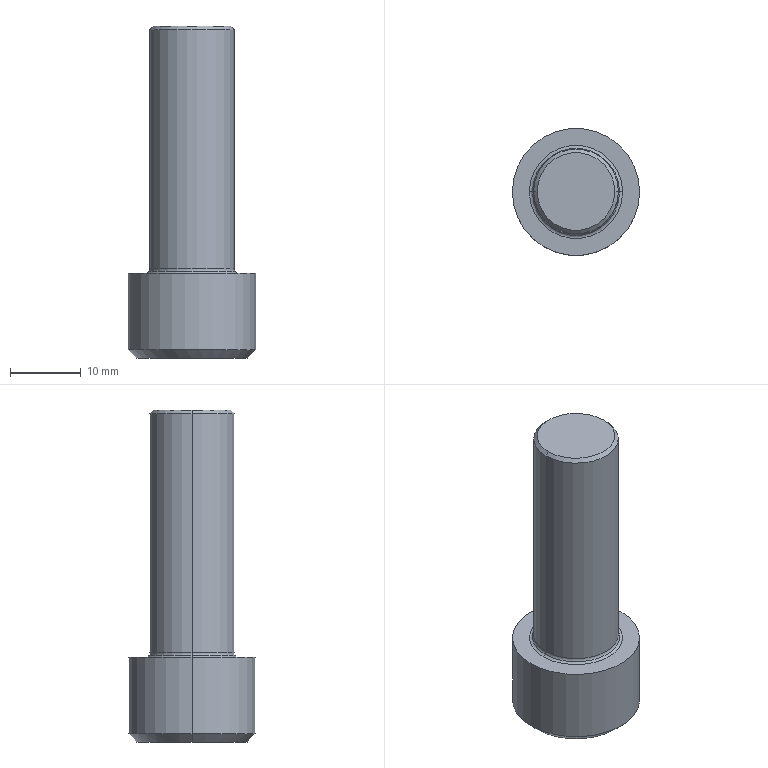Part | Creo | 1 solid | 23 faces | box 18 x 18 x 47 mm | volume 6339 mm3 | plane 9 | cone 6 | cylinder 4 | torus 4 | commonest cylinder face diameters 12 x2 18 x2
STEP:
#1=CARTESIAN_POINT('',(0.,0.,0.));
#2=DIRECTION('',(0.,0.,1.));
#3=DIRECTION('',(1.,0.,0.));
#4=AXIS2_PLACEMENT_3D('',#1,#2,#3);
#5=CARTESIAN_POINT('',(61.475,-67.,-247.5));
#6=VERTEX_POINT('',#5);
#7=CARTESIAN_POINT('',(64.361,-62.,-247.5));
#8=VERTEX_POINT('',#7);
#9=CARTESIAN_POINT('',(61.475,-67.,-247.5));
#10=CARTESIAN_POINT('',(61.609,-66.767,-247.422));
#11=CARTESIAN_POINT('',(61.88,-66.298,-247.282));
#12=CARTESIAN_POINT('',(62.291,-65.586,-247.131));
#13=CARTESIAN_POINT('',(62.707,-64.865,-247.05));
#14=CARTESIAN_POINT('',(63.127,-64.137,-247.05));
#15=CARTESIAN_POINT('',(63.544,-63.416,-247.131));
#16=CARTESIAN_POINT('',(63.955,-62.704,-247.282));
#17=CARTESIAN_POINT('',(64.226,-62.234,-247.422));
#18=CARTESIAN_POINT('',(64.361,-62.,-247.5));
#19=B_SPLINE_CURVE_WITH_KNOTS('',3,(#9,#10,#11,#12,#13,#14,#15,#16,#17,#18),.UNSPECIFIED.,.F.,.F.,(4,1,1,1,1,1,1,4),(0.,0.1429,0.2857,0.4286,0.5714,0.7143,0.8571,1.),.UNSPECIFIED.);
#20=EDGE_CURVE('',#6,#8,#19,.T.);
#21=ORIENTED_EDGE('',*,*,#20,.F.);
#22=CARTESIAN_POINT('',(67.248,-67.,-244.167));
#23=VERTEX_POINT('',#22);
#24=CARTESIAN_POINT('',(67.248,-67.,-244.167));
#25=DIRECTION('',(-0.866,0.,-0.5));
#26=VECTOR('',#25,6.667);
#27=LINE('',#24,#26);
#28=EDGE_CURVE('',#23,#6,#27,.T.);
#29=ORIENTED_EDGE('',*,*,#28,.F.);
#30=CARTESIAN_POINT('',(73.022,-67.,-247.5));
#31=VERTEX_POINT('',#30);
#32=CARTESIAN_POINT('',(67.248,-67.,-244.167));
#33=DIRECTION('',(0.866,0.,-0.5));
#34=VECTOR('',#33,6.667);
#35=LINE('',#32,#34);
#36=EDGE_CURVE('',#23,#31,#35,.T.);
#37=ORIENTED_EDGE('',*,*,#36,.T.);
#38=CARTESIAN_POINT('',(70.135,-62.,-247.5));
#39=VERTEX_POINT('',#38);
#40=CARTESIAN_POINT('',(70.135,-62.,-247.5));
#41=CARTESIAN_POINT('',(70.269,-62.233,-247.422));
#42=CARTESIAN_POINT('',(70.54,-62.702,-247.282));
#43=CARTESIAN_POINT('',(70.951,-63.414,-247.131));
#44=CARTESIAN_POINT('',(71.367,-64.135,-247.05));
#45=CARTESIAN_POINT('',(71.788,-64.863,-247.05));
#46=CARTESIAN_POINT('',(72.204,-65.584,-247.131));
#47=CARTESIAN_POINT('',(72.615,-66.296,-247.282));
#48=CARTESIAN_POINT('',(72.886,-66.766,-247.422));
#49=CARTESIAN_POINT('',(73.022,-67.,-247.5));
#50=B_SPLINE_CURVE_WITH_KNOTS('',3,(#40,#41,#42,#43,#44,#45,#46,#47,#48,#49),.UNSPECIFIED.,.F.,.F.,(4,1,1,1,1,1,1,4),(0.,0.1429,0.2857,0.4286,0.5714,0.7143,0.8571,1.),.UNSPECIFIED.);
#51=EDGE_CURVE('',#39,#31,#50,.T.);
#52=ORIENTED_EDGE('',*,*,#51,.F.);
#53=CARTESIAN_POINT('',(64.361,-62.,-247.5));
#54=CARTESIAN_POINT('',(64.629,-62.,-247.423));
#55=CARTESIAN_POINT('',(65.167,-62.,-247.283));
#56=CARTESIAN_POINT('',(65.993,-62.,-247.131));
#57=CARTESIAN_POINT('',(66.829,-62.,-247.05));
#58=CARTESIAN_POINT('',(67.664,-62.,-247.05));
#59=CARTESIAN_POINT('',(68.498,-62.,-247.13));
#60=CARTESIAN_POINT('',(69.325,-62.,-247.282));
#61=CARTESIAN_POINT('',(69.866,-62.,-247.422));
#62=CARTESIAN_POINT('',(70.135,-62.,-247.5));
#63=B_SPLINE_CURVE_WITH_KNOTS('',3,(#53,#54,#55,#56,#57,#58,#59,#60,#61,#62),.UNSPECIFIED.,.F.,.F.,(4,1,1,1,1,1,1,4),(0.,0.1429,0.2857,0.4286,0.5714,0.7143,0.8571,1.),.UNSPECIFIED.);
#64=EDGE_CURVE('',#8,#39,#63,.T.);
#65=ORIENTED_EDGE('',*,*,#64,.F.);
#66=EDGE_LOOP('',(#21,#29,#37,#52,#65));
#67=FACE_OUTER_BOUND('',#66,.F.);
#68=CARTESIAN_POINT('',(67.248,-67.,-245.867));
#69=DIRECTION('',(0.,0.,-1.));
#70=DIRECTION('',(-1.,0.,0.));
#71=AXIS2_PLACEMENT_3D('',#68,#69,#70);
#72=CONICAL_SURFACE('',#71,2.944,60.);
#73=ADVANCED_FACE('',(#67),#72,.F.);
#74=CARTESIAN_POINT('',(64.361,-62.,-253.5));
#75=VERTEX_POINT('',#74);
#76=CARTESIAN_POINT('',(61.475,-67.,-253.5));
#77=VERTEX_POINT('',#76);
#78=CARTESIAN_POINT('',(64.361,-62.,-253.5));
#79=DIRECTION('',(-0.5,-0.866,0.));
#80=VECTOR('',#79,5.774);
#81=LINE('',#78,#80);
#82=EDGE_CURVE('',#75,#77,#81,.T.);
#83=ORIENTED_EDGE('',*,*,#82,.T.);
#84=CARTESIAN_POINT('',(61.475,-67.,-253.5));
#85=DIRECTION('',(0.,0.,1.));
#86=VECTOR('',#85,6.);
#87=LINE('',#84,#86);
#88=EDGE_CURVE('',#77,#6,#87,.T.);
#89=ORIENTED_EDGE('',*,*,#88,.T.);
#90=ORIENTED_EDGE('',*,*,#20,.T.);
#91=CARTESIAN_POINT('',(64.361,-62.,-253.5));
#92=DIRECTION('',(0.,0.,1.));
#93=VECTOR('',#92,6.);
#94=LINE('',#91,#93);
#95=EDGE_CURVE('',#75,#8,#94,.T.);
#96=ORIENTED_EDGE('',*,*,#95,.F.);
#97=EDGE_LOOP('',(#83,#89,#90,#96));
#98=FACE_OUTER_BOUND('',#97,.F.);
#99=CARTESIAN_POINT('',(64.361,-62.,-247.5));
#100=DIRECTION('',(0.866,-0.5,0.));
#101=DIRECTION('',(-0.5,-0.866,0.));
#102=AXIS2_PLACEMENT_3D('',#99,#100,#101);
#103=PLANE('',#102);
#104=ADVANCED_FACE('',(#98),#103,.T.);
#105=CARTESIAN_POINT('',(59.448,-67.,-253.5));
#106=VERTEX_POINT('',#105);
#107=CARTESIAN_POINT('',(75.048,-67.,-253.5));
#108=VERTEX_POINT('',#107);
#109=CARTESIAN_POINT('',(67.248,-67.,-253.5));
#110=DIRECTION('',(0.,0.,-1.));
#111=DIRECTION('',(-1.,0.,0.));
#112=AXIS2_PLACEMENT_3D('',#109,#110,#111);
#113=CIRCLE('',#112,7.8);
#114=EDGE_CURVE('',#106,#108,#113,.T.);
#115=ORIENTED_EDGE('',*,*,#114,.F.);
#116=CARTESIAN_POINT('',(67.248,-67.,-253.5));
#117=DIRECTION('',(0.,0.,-1.));
#118=DIRECTION('',(1.,0.,0.));
#119=AXIS2_PLACEMENT_3D('',#116,#117,#118);
#120=CIRCLE('',#119,7.8);
#121=EDGE_CURVE('',#108,#106,#120,.T.);
#122=ORIENTED_EDGE('',*,*,#121,.F.);
#123=EDGE_LOOP('',(#115,#122));
#124=FACE_OUTER_BOUND('',#123,.F.);
#125=CARTESIAN_POINT('',(64.361,-72.,-253.5));
#126=VERTEX_POINT('',#125);
#127=CARTESIAN_POINT('',(61.475,-67.,-253.5));
#128=DIRECTION('',(0.5,-0.866,0.));
#129=VECTOR('',#128,5.774);
#130=LINE('',#127,#129);
#131=EDGE_CURVE('',#77,#126,#130,.T.);
#132=ORIENTED_EDGE('',*,*,#131,.F.);
#133=ORIENTED_EDGE('',*,*,#82,.F.);
#134=CARTESIAN_POINT('',(70.135,-62.,-253.5));
#135=VERTEX_POINT('',#134);
#136=CARTESIAN_POINT('',(64.361,-62.,-253.5));
#137=DIRECTION('',(1.,0.,0.));
#138=VECTOR('',#137,5.774);
#139=LINE('',#136,#138);
#140=EDGE_CURVE('',#75,#135,#139,.T.);
#141=ORIENTED_EDGE('',*,*,#140,.T.);
#142=CARTESIAN_POINT('',(73.022,-67.,-253.5));
#143=VERTEX_POINT('',#142);
#144=CARTESIAN_POINT('',(73.022,-67.,-253.5));
#145=DIRECTION('',(-0.5,0.866,0.));
#146=VECTOR('',#145,5.774);
#147=LINE('',#144,#146);
#148=EDGE_CURVE('',#143,#135,#147,.T.);
#149=ORIENTED_EDGE('',*,*,#148,.F.);
#150=CARTESIAN_POINT('',(70.135,-72.,-253.5));
#151=VERTEX_POINT('',#150);
#152=CARTESIAN_POINT('',(70.135,-72.,-253.5));
#153=DIRECTION('',(0.5,0.866,0.));
#154=VECTOR('',#153,5.774);
#155=LINE('',#152,#154);
#156=EDGE_CURVE('',#151,#143,#155,.T.);
#157=ORIENTED_EDGE('',*,*,#156,.F.);
#158=CARTESIAN_POINT('',(70.135,-72.,-253.5));
#159=DIRECTION('',(-1.,0.,0.));
#160=VECTOR('',#159,5.774);
#161=LINE('',#158,#160);
#162=EDGE_CURVE('',#151,#126,#161,.T.);
#163=ORIENTED_EDGE('',*,*,#162,.T.);
#164=EDGE_LOOP('',(#132,#133,#141,#149,#157,#163));
#165=FACE_BOUND('',#164,.F.);
#166=CARTESIAN_POINT('',(67.248,-67.,-253.5));
#167=DIRECTION('',(0.,0.,-1.));
#168=DIRECTION('',(-1.,0.,0.));
#169=AXIS2_PLACEMENT_3D('',#166,#167,#168);
#170=PLANE('',#169);
#171=ADVANCED_FACE('',(#124,#165),#170,.T.);
#172=CARTESIAN_POINT('',(58.248,-67.,-252.3));
#173=VERTEX_POINT('',#172);
#174=CARTESIAN_POINT('',(76.248,-67.,-252.3));
#175=VERTEX_POINT('',#174);
#176=CARTESIAN_POINT('',(67.248,-67.,-252.3));
#177=DIRECTION('',(0.,0.,-1.));
#178=DIRECTION('',(-1.,0.,0.));
#179=AXIS2_PLACEMENT_3D('',#176,#177,#178);
#180=CIRCLE('',#179,9.);
#181=EDGE_CURVE('',#173,#175,#180,.T.);
#182=ORIENTED_EDGE('',*,*,#181,.F.);
#183=CARTESIAN_POINT('',(59.448,-67.,-253.5));
#184=DIRECTION('',(-0.7071,0.,0.7071));
#185=VECTOR('',#184,1.697);
#186=LINE('',#183,#185);
#187=EDGE_CURVE('',#106,#173,#186,.T.);
#188=ORIENTED_EDGE('',*,*,#187,.F.);
#189=ORIENTED_EDGE('',*,*,#114,.T.);
#190=CARTESIAN_POINT('',(75.048,-67.,-253.5));
#191=DIRECTION('',(0.7071,0.,0.7071));
#192=VECTOR('',#191,1.697);
#193=LINE('',#190,#192);
#194=EDGE_CURVE('',#108,#175,#193,.T.);
#195=ORIENTED_EDGE('',*,*,#194,.T.);
#196=EDGE_LOOP('',(#182,#188,#189,#195));
#197=FACE_OUTER_BOUND('',#196,.F.);
#198=CARTESIAN_POINT('',(67.248,-67.,-252.9));
#199=DIRECTION('',(0.,0.,1.));
#200=DIRECTION('',(1.,0.,0.));
#201=AXIS2_PLACEMENT_3D('',#198,#199,#200);
#202=CONICAL_SURFACE('',#201,8.4,45.);
#203=ADVANCED_FACE('',(#197),#202,.T.);
#204=ORIENTED_EDGE('',*,*,#181,.T.);
#205=CARTESIAN_POINT('',(76.248,-67.,-241.5));
#206=VERTEX_POINT('',#205);
#207=CARTESIAN_POINT('',(76.248,-67.,-241.5));
#208=DIRECTION('',(0.,0.,-1.));
#209=VECTOR('',#208,10.8);
#210=LINE('',#207,#209);
#211=EDGE_CURVE('',#206,#175,#210,.T.);
#212=ORIENTED_EDGE('',*,*,#211,.F.);
#213=CARTESIAN_POINT('',(58.248,-67.,-241.5));
#214=VERTEX_POINT('',#213);
#215=CARTESIAN_POINT('',(67.248,-67.,-241.5));
#216=DIRECTION('',(0.,0.,1.));
#217=DIRECTION('',(1.,0.,0.));
#218=AXIS2_PLACEMENT_3D('',#215,#216,#217);
#219=CIRCLE('',#218,9.);
#220=EDGE_CURVE('',#206,#214,#219,.T.);
#221=ORIENTED_EDGE('',*,*,#220,.T.);
#222=CARTESIAN_POINT('',(58.248,-67.,-241.5));
#223=DIRECTION('',(0.,0.,-1.));
#224=VECTOR('',#223,10.8);
#225=LINE('',#222,#224);
#226=EDGE_CURVE('',#214,#173,#225,.T.);
#227=ORIENTED_EDGE('',*,*,#226,.T.);
#228=EDGE_LOOP('',(#204,#212,#221,#227));
#229=FACE_OUTER_BOUND('',#228,.F.);
#230=CARTESIAN_POINT('',(67.248,-67.,-241.5));
#231=DIRECTION('',(0.,0.,-1.));
#232=DIRECTION('',(-1.,0.,0.));
#233=AXIS2_PLACEMENT_3D('',#230,#231,#232);
#234=CYLINDRICAL_SURFACE('',#233,9.);
#235=ADVANCED_FACE('',(#229),#234,.T.);
#236=CARTESIAN_POINT('',(67.248,-67.,-252.3));
#237=DIRECTION('',(0.,0.,-1.));
#238=DIRECTION('',(1.,0.,0.));
#239=AXIS2_PLACEMENT_3D('',#236,#237,#238);
#240=CIRCLE('',#239,9.);
#241=EDGE_CURVE('',#175,#173,#240,.T.);
#242=ORIENTED_EDGE('',*,*,#241,.T.);
#243=ORIENTED_EDGE('',*,*,#226,.F.);
#244=CARTESIAN_POINT('',(67.248,-67.,-241.5));
#245=DIRECTION('',(0.,0.,1.));
#246=DIRECTION('',(-1.,0.,0.));
#247=AXIS2_PLACEMENT_3D('',#244,#245,#246);
#248=CIRCLE('',#247,9.);
#249=EDGE_CURVE('',#214,#206,#248,.T.);
#250=ORIENTED_EDGE('',*,*,#249,.T.);
#251=ORIENTED_EDGE('',*,*,#211,.T.);
#252=EDGE_LOOP('',(#242,#243,#250,#251));
#253=FACE_OUTER_BOUND('',#252,.F.);
#254=CARTESIAN_POINT('',(67.248,-67.,-241.5));
#255=DIRECTION('',(0.,0.,-1.));
#256=DIRECTION('',(-1.,0.,0.));
#257=AXIS2_PLACEMENT_3D('',#254,#255,#256);
#258=CYLINDRICAL_SURFACE('',#257,9.);
#259=ADVANCED_FACE('',(#253),#258,.T.);
#260=ORIENTED_EDGE('',*,*,#241,.F.);
#261=ORIENTED_EDGE('',*,*,#194,.F.);
#262=ORIENTED_EDGE('',*,*,#121,.T.);
#263=ORIENTED_EDGE('',*,*,#187,.T.);
#264=EDGE_LOOP('',(#260,#261,#262,#263));
#265=FACE_OUTER_BOUND('',#264,.F.);
#266=CARTESIAN_POINT('',(67.248,-67.,-252.9));
#267=DIRECTION('',(0.,0.,1.));
#268=DIRECTION('',(1.,0.,0.));
#269=AXIS2_PLACEMENT_3D('',#266,#267,#268);
#270=CONICAL_SURFACE('',#269,8.4,45.);
#271=ADVANCED_FACE('',(#265),#270,.T.);
#272=ORIENTED_EDGE('',*,*,#249,.F.);
#273=ORIENTED_EDGE('',*,*,#220,.F.);
#274=EDGE_LOOP('',(#272,#273));
#275=FACE_OUTER_BOUND('',#274,.F.);
#276=CARTESIAN_POINT('',(60.648,-67.,-241.5));
#277=VERTEX_POINT('',#276);
#278=CARTESIAN_POINT('',(73.848,-67.,-241.5));
#279=VERTEX_POINT('',#278);
#280=CARTESIAN_POINT('',(67.248,-67.,-241.5));
#281=DIRECTION('',(0.,0.,-1.));
#282=DIRECTION('',(-1.,0.,0.));
#283=AXIS2_PLACEMENT_3D('',#280,#281,#282);
#284=CIRCLE('',#283,6.6);
#285=EDGE_CURVE('',#277,#279,#284,.T.);
#286=ORIENTED_EDGE('',*,*,#285,.F.);
#287=CARTESIAN_POINT('',(67.248,-67.,-241.5));
#288=DIRECTION('',(0.,0.,-1.));
#289=DIRECTION('',(1.,0.,0.));
#290=AXIS2_PLACEMENT_3D('',#287,#288,#289);
#291=CIRCLE('',#290,6.6);
#292=EDGE_CURVE('',#279,#277,#291,.T.);
#293=ORIENTED_EDGE('',*,*,#292,.F.);
#294=EDGE_LOOP('',(#286,#293));
#295=FACE_BOUND('',#294,.F.);
#296=CARTESIAN_POINT('',(67.248,-67.,-241.5));
#297=DIRECTION('',(0.,0.,-1.));
#298=DIRECTION('',(-1.,0.,0.));
#299=AXIS2_PLACEMENT_3D('',#296,#297,#298);
#300=PLANE('',#299);
#301=ADVANCED_FACE('',(#275,#295),#300,.F.);
#302=ORIENTED_EDGE('',*,*,#285,.T.);
#303=CARTESIAN_POINT('',(73.424,-67.,-241.324));
#304=VERTEX_POINT('',#303);
#305=CARTESIAN_POINT('',(73.848,-67.,-240.9));
#306=DIRECTION('',(0.,1.,0.));
#307=DIRECTION('',(0.,0.,-1.));
#308=AXIS2_PLACEMENT_3D('',#305,#306,#307);
#309=CIRCLE('',#308,0.6);
#310=EDGE_CURVE('',#279,#304,#309,.T.);
#311=ORIENTED_EDGE('',*,*,#310,.T.);
#312=CARTESIAN_POINT('',(61.072,-67.,-241.324));
#313=VERTEX_POINT('',#312);
#314=CARTESIAN_POINT('',(67.248,-67.,-241.324));
#315=DIRECTION('',(0.,0.,-1.));
#316=DIRECTION('',(-1.,0.,0.));
#317=AXIS2_PLACEMENT_3D('',#314,#315,#316);
#318=CIRCLE('',#317,6.176);
#319=EDGE_CURVE('',#313,#304,#318,.T.);
#320=ORIENTED_EDGE('',*,*,#319,.F.);
#321=CARTESIAN_POINT('',(60.648,-67.,-240.9));
#322=DIRECTION('',(0.,-1.,0.));
#323=DIRECTION('',(0.,0.,-1.));
#324=AXIS2_PLACEMENT_3D('',#321,#322,#323);
#325=CIRCLE('',#324,0.6);
#326=EDGE_CURVE('',#277,#313,#325,.T.);
#327=ORIENTED_EDGE('',*,*,#326,.F.);
#328=EDGE_LOOP('',(#302,#311,#320,#327));
#329=FACE_OUTER_BOUND('',#328,.F.);
#330=CARTESIAN_POINT('',(67.248,-67.,-240.9));
#331=DIRECTION('',(0.,0.,-1.));
#332=DIRECTION('',(-1.,0.,0.));
#333=AXIS2_PLACEMENT_3D('',#330,#331,#332);
#334=TOROIDAL_SURFACE('',#333,6.6,0.6);
#335=ADVANCED_FACE('',(#329),#334,.F.);
#336=ORIENTED_EDGE('',*,*,#292,.T.);
#337=ORIENTED_EDGE('',*,*,#326,.T.);
#338=CARTESIAN_POINT('',(67.248,-67.,-241.324));
#339=DIRECTION('',(0.,0.,-1.));
#340=DIRECTION('',(1.,0.,0.));
#341=AXIS2_PLACEMENT_3D('',#338,#339,#340);
#342=CIRCLE('',#341,6.176);
#343=EDGE_CURVE('',#304,#313,#342,.T.);
#344=ORIENTED_EDGE('',*,*,#343,.F.);
#345=ORIENTED_EDGE('',*,*,#310,.F.);
#346=EDGE_LOOP('',(#336,#337,#344,#345));
#347=FACE_OUTER_BOUND('',#346,.F.);
#348=CARTESIAN_POINT('',(67.248,-67.,-240.9));
#349=DIRECTION('',(0.,0.,-1.));
#350=DIRECTION('',(-1.,0.,0.));
#351=AXIS2_PLACEMENT_3D('',#348,#349,#350);
#352=TOROIDAL_SURFACE('',#351,6.6,0.6);
#353=ADVANCED_FACE('',(#347),#352,.F.);
#354=CARTESIAN_POINT('',(73.248,-67.,-240.9));
#355=VERTEX_POINT('',#354);
#356=CARTESIAN_POINT('',(61.248,-67.,-240.9));
#357=VERTEX_POINT('',#356);
#358=CARTESIAN_POINT('',(67.248,-67.,-240.9));
#359=DIRECTION('',(0.,0.,-1.));
#360=DIRECTION('',(1.,0.,0.));
#361=AXIS2_PLACEMENT_3D('',#358,#359,#360);
#362=CIRCLE('',#361,6.);
#363=EDGE_CURVE('',#355,#357,#362,.T.);
#364=ORIENTED_EDGE('',*,*,#363,.F.);
#365=CARTESIAN_POINT('',(73.848,-67.,-240.9));
#366=DIRECTION('',(0.,1.,0.));
#367=DIRECTION('',(-0.7071,0.,-0.7071));
#368=AXIS2_PLACEMENT_3D('',#365,#366,#367);
#369=CIRCLE('',#368,0.6);
#370=EDGE_CURVE('',#304,#355,#369,.T.);
#371=ORIENTED_EDGE('',*,*,#370,.F.);
#372=ORIENTED_EDGE('',*,*,#343,.T.);
#373=CARTESIAN_POINT('',(60.648,-67.,-240.9));
#374=DIRECTION('',(0.,-1.,0.));
#375=DIRECTION('',(0.7071,0.,-0.7071));
#376=AXIS2_PLACEMENT_3D('',#373,#374,#375);
#377=CIRCLE('',#376,0.6);
#378=EDGE_CURVE('',#313,#357,#377,.T.);
#379=ORIENTED_EDGE('',*,*,#378,.T.);
#380=EDGE_LOOP('',(#364,#371,#372,#379));
#381=FACE_OUTER_BOUND('',#380,.F.);
#382=CARTESIAN_POINT('',(67.248,-67.,-240.9));
#383=DIRECTION('',(0.,0.,-1.));
#384=DIRECTION('',(-1.,0.,0.));
#385=AXIS2_PLACEMENT_3D('',#382,#383,#384);
#386=TOROIDAL_SURFACE('',#385,6.6,0.6);
#387=ADVANCED_FACE('',(#381),#386,.F.);
#388=CARTESIAN_POINT('',(61.248,-67.,-207.));
#389=VERTEX_POINT('',#388);
#390=CARTESIAN_POINT('',(73.248,-67.,-207.));
#391=VERTEX_POINT('',#390);
#392=CARTESIAN_POINT('',(67.248,-67.,-207.));
#393=DIRECTION('',(0.,0.,1.));
#394=DIRECTION('',(-1.,0.,0.));
#395=AXIS2_PLACEMENT_3D('',#392,#393,#394);
#396=CIRCLE('',#395,6.);
#397=EDGE_CURVE('',#389,#391,#396,.T.);
#398=ORIENTED_EDGE('',*,*,#397,.T.);
#399=CARTESIAN_POINT('',(73.248,-67.,-207.));
#400=DIRECTION('',(0.,0.,-1.));
#401=VECTOR('',#400,33.9);
#402=LINE('',#399,#401);
#403=EDGE_CURVE('',#391,#355,#402,.T.);
#404=ORIENTED_EDGE('',*,*,#403,.T.);
#405=ORIENTED_EDGE('',*,*,#363,.T.);
#406=CARTESIAN_POINT('',(61.248,-67.,-207.));
#407=DIRECTION('',(0.,0.,-1.));
#408=VECTOR('',#407,33.9);
#409=LINE('',#406,#408);
#410=EDGE_CURVE('',#389,#357,#409,.T.);
#411=ORIENTED_EDGE('',*,*,#410,.F.);
#412=EDGE_LOOP('',(#398,#404,#405,#411));
#413=FACE_OUTER_BOUND('',#412,.F.);
#414=CARTESIAN_POINT('',(67.248,-67.,-206.5));
#415=DIRECTION('',(0.,0.,-1.));
#416=DIRECTION('',(-1.,0.,0.));
#417=AXIS2_PLACEMENT_3D('',#414,#415,#416);
#418=CYLINDRICAL_SURFACE('',#417,6.);
#419=ADVANCED_FACE('',(#413),#418,.T.);
#420=CARTESIAN_POINT('',(61.748,-67.,-206.5));
#421=VERTEX_POINT('',#420);
#422=CARTESIAN_POINT('',(72.748,-67.,-206.5));
#423=VERTEX_POINT('',#422);
#424=CARTESIAN_POINT('',(67.248,-67.,-206.5));
#425=DIRECTION('',(0.,0.,1.));
#426=DIRECTION('',(-1.,0.,0.));
#427=AXIS2_PLACEMENT_3D('',#424,#425,#426);
#428=CIRCLE('',#427,5.5);
#429=EDGE_CURVE('',#421,#423,#428,.T.);
#430=ORIENTED_EDGE('',*,*,#429,.T.);
#431=CARTESIAN_POINT('',(72.748,-67.,-206.5));
#432=DIRECTION('',(0.7071,0.,-0.7071));
#433=VECTOR('',#432,0.7071);
#434=LINE('',#431,#433);
#435=EDGE_CURVE('',#423,#391,#434,.T.);
#436=ORIENTED_EDGE('',*,*,#435,.T.);
#437=ORIENTED_EDGE('',*,*,#397,.F.);
#438=CARTESIAN_POINT('',(61.748,-67.,-206.5));
#439=DIRECTION('',(-0.7071,0.,-0.7071));
#440=VECTOR('',#439,0.7071);
#441=LINE('',#438,#440);
#442=EDGE_CURVE('',#421,#389,#441,.T.);
#443=ORIENTED_EDGE('',*,*,#442,.F.);
#444=EDGE_LOOP('',(#430,#436,#437,#443));
#445=FACE_OUTER_BOUND('',#444,.F.);
#446=CARTESIAN_POINT('',(67.248,-67.,-206.75));
#447=DIRECTION('',(0.,0.,-1.));
#448=DIRECTION('',(-1.,0.,0.));
#449=AXIS2_PLACEMENT_3D('',#446,#447,#448);
#450=CONICAL_SURFACE('',#449,5.75,45.);
#451=ADVANCED_FACE('',(#445),#450,.T.);
#452=ORIENTED_EDGE('',*,*,#429,.F.);
#453=CARTESIAN_POINT('',(67.248,-67.,-206.5));
#454=DIRECTION('',(0.,0.,1.));
#455=DIRECTION('',(1.,0.,0.));
#456=AXIS2_PLACEMENT_3D('',#453,#454,#455);
#457=CIRCLE('',#456,5.5);
#458=EDGE_CURVE('',#423,#421,#457,.T.);
#459=ORIENTED_EDGE('',*,*,#458,.F.);
#460=EDGE_LOOP('',(#452,#459));
#461=FACE_OUTER_BOUND('',#460,.F.);
#462=CARTESIAN_POINT('',(67.248,-67.,-206.5));
#463=DIRECTION('',(0.,0.,-1.));
#464=DIRECTION('',(-1.,0.,0.));
#465=AXIS2_PLACEMENT_3D('',#462,#463,#464);
#466=PLANE('',#465);
#467=ADVANCED_FACE('',(#461),#466,.F.);
#468=ORIENTED_EDGE('',*,*,#458,.T.);
#469=ORIENTED_EDGE('',*,*,#442,.T.);
#470=CARTESIAN_POINT('',(67.248,-67.,-207.));
#471=DIRECTION('',(0.,0.,1.));
#472=DIRECTION('',(1.,0.,0.));
#473=AXIS2_PLACEMENT_3D('',#470,#471,#472);
#474=CIRCLE('',#473,6.);
#475=EDGE_CURVE('',#391,#389,#474,.T.);
#476=ORIENTED_EDGE('',*,*,#475,.F.);
#477=ORIENTED_EDGE('',*,*,#435,.F.);
#478=EDGE_LOOP('',(#468,#469,#476,#477));
#479=FACE_OUTER_BOUND('',#478,.F.);
#480=CARTESIAN_POINT('',(67.248,-67.,-206.75));
#481=DIRECTION('',(0.,0.,-1.));
#482=DIRECTION('',(-1.,0.,0.));
#483=AXIS2_PLACEMENT_3D('',#480,#481,#482);
#484=CONICAL_SURFACE('',#483,5.75,45.);
#485=ADVANCED_FACE('',(#479),#484,.T.);
#486=ORIENTED_EDGE('',*,*,#475,.T.);
#487=ORIENTED_EDGE('',*,*,#410,.T.);
#488=CARTESIAN_POINT('',(67.248,-67.,-240.9));
#489=DIRECTION('',(0.,0.,-1.));
#490=DIRECTION('',(-1.,0.,0.));
#491=AXIS2_PLACEMENT_3D('',#488,#489,#490);
#492=CIRCLE('',#491,6.);
#493=EDGE_CURVE('',#357,#355,#492,.T.);
#494=ORIENTED_EDGE('',*,*,#493,.T.);
#495=ORIENTED_EDGE('',*,*,#403,.F.);
#496=EDGE_LOOP('',(#486,#487,#494,#495));
#497=FACE_OUTER_BOUND('',#496,.F.);
#498=CARTESIAN_POINT('',(67.248,-67.,-206.5));
#499=DIRECTION('',(0.,0.,-1.));
#500=DIRECTION('',(-1.,0.,0.));
#501=AXIS2_PLACEMENT_3D('',#498,#499,#500);
#502=CYLINDRICAL_SURFACE('',#501,6.);
#503=ADVANCED_FACE('',(#497),#502,.T.);
#504=ORIENTED_EDGE('',*,*,#493,.F.);
#505=ORIENTED_EDGE('',*,*,#378,.F.);
#506=ORIENTED_EDGE('',*,*,#319,.T.);
#507=ORIENTED_EDGE('',*,*,#370,.T.);
#508=EDGE_LOOP('',(#504,#505,#506,#507));
#509=FACE_OUTER_BOUND('',#508,.F.);
#510=CARTESIAN_POINT('',(67.248,-67.,-240.9));
#511=DIRECTION('',(0.,0.,-1.));
#512=DIRECTION('',(-1.,0.,0.));
#513=AXIS2_PLACEMENT_3D('',#510,#511,#512);
#514=TOROIDAL_SURFACE('',#513,6.6,0.6);
#515=ADVANCED_FACE('',(#509),#514,.F.);
#516=ORIENTED_EDGE('',*,*,#131,.T.);
#517=CARTESIAN_POINT('',(64.361,-72.,-247.5));
#518=VERTEX_POINT('',#517);
#519=CARTESIAN_POINT('',(64.361,-72.,-253.5));
#520=DIRECTION('',(0.,0.,1.));
#521=VECTOR('',#520,6.);
#522=LINE('',#519,#521);
#523=EDGE_CURVE('',#126,#518,#522,.T.);
#524=ORIENTED_EDGE('',*,*,#523,.T.);
#525=CARTESIAN_POINT('',(64.361,-72.,-247.5));
#526=CARTESIAN_POINT('',(64.227,-71.767,-247.422));
#527=CARTESIAN_POINT('',(63.956,-71.298,-247.282));
#528=CARTESIAN_POINT('',(63.545,-70.586,-247.131));
#529=CARTESIAN_POINT('',(63.129,-69.865,-247.05));
#530=CARTESIAN_POINT('',(62.708,-69.137,-247.05));
#531=CARTESIAN_POINT('',(62.292,-68.416,-247.131));
#532=CARTESIAN_POINT('',(61.881,-67.704,-247.282));
#533=CARTESIAN_POINT('',(61.61,-67.234,-247.422));
#534=CARTESIAN_POINT('',(61.475,-67.,-247.5));
#535=B_SPLINE_CURVE_WITH_KNOTS('',3,(#525,#526,#527,#528,#529,#530,#531,#532,#533,#534),.UNSPECIFIED.,.F.,.F.,(4,1,1,1,1,1,1,4),(0.,0.1429,0.2857,0.4286,0.5714,0.7143,0.8571,1.),.UNSPECIFIED.);
#536=EDGE_CURVE('',#518,#6,#535,.T.);
#537=ORIENTED_EDGE('',*,*,#536,.T.);
#538=ORIENTED_EDGE('',*,*,#88,.F.);
#539=EDGE_LOOP('',(#516,#524,#537,#538));
#540=FACE_OUTER_BOUND('',#539,.F.);
#541=CARTESIAN_POINT('',(61.475,-67.,-247.5));
#542=DIRECTION('',(0.866,0.5,0.));
#543=DIRECTION('',(0.5,-0.866,0.));
#544=AXIS2_PLACEMENT_3D('',#541,#542,#543);
#545=PLANE('',#544);
#546=ADVANCED_FACE('',(#540),#545,.T.);
#547=ORIENTED_EDGE('',*,*,#162,.F.);
#548=CARTESIAN_POINT('',(70.135,-72.,-247.5));
#549=VERTEX_POINT('',#548);
#550=CARTESIAN_POINT('',(70.135,-72.,-253.5));
#551=DIRECTION('',(0.,0.,1.));
#552=VECTOR('',#551,6.);
#553=LINE('',#550,#552);
#554=EDGE_CURVE('',#151,#549,#553,.T.);
#555=ORIENTED_EDGE('',*,*,#554,.T.);
#556=CARTESIAN_POINT('',(70.135,-72.,-247.5));
#557=CARTESIAN_POINT('',(69.866,-72.,-247.422));
#558=CARTESIAN_POINT('',(69.325,-72.,-247.282));
#559=CARTESIAN_POINT('',(68.498,-72.,-247.13));
#560=CARTESIAN_POINT('',(67.664,-72.,-247.05));
#561=CARTESIAN_POINT('',(66.829,-72.,-247.05));
#562=CARTESIAN_POINT('',(65.993,-72.,-247.131));
#563=CARTESIAN_POINT('',(65.167,-72.,-247.283));
#564=CARTESIAN_POINT('',(64.629,-72.,-247.423));
#565=CARTESIAN_POINT('',(64.361,-72.,-247.5));
#566=B_SPLINE_CURVE_WITH_KNOTS('',3,(#556,#557,#558,#559,#560,#561,#562,#563,#564,#565),.UNSPECIFIED.,.F.,.F.,(4,1,1,1,1,1,1,4),(0.,0.1429,0.2857,0.4286,0.5714,0.7143,0.8571,1.),.UNSPECIFIED.);
#567=EDGE_CURVE('',#549,#518,#566,.T.);
#568=ORIENTED_EDGE('',*,*,#567,.T.);
#569=ORIENTED_EDGE('',*,*,#523,.F.);
#570=EDGE_LOOP('',(#547,#555,#568,#569));
#571=FACE_OUTER_BOUND('',#570,.F.);
#572=CARTESIAN_POINT('',(64.361,-72.,-247.5));
#573=DIRECTION('',(0.,1.,0.));
#574=DIRECTION('',(0.,0.,-1.));
#575=AXIS2_PLACEMENT_3D('',#572,#573,#574);
#576=PLANE('',#575);
#577=ADVANCED_FACE('',(#571),#576,.T.);
#578=ORIENTED_EDGE('',*,*,#156,.T.);
#579=CARTESIAN_POINT('',(73.022,-67.,-253.5));
#580=DIRECTION('',(0.,0.,1.));
#581=VECTOR('',#580,6.);
#582=LINE('',#579,#581);
#583=EDGE_CURVE('',#143,#31,#582,.T.);
#584=ORIENTED_EDGE('',*,*,#583,.T.);
#585=CARTESIAN_POINT('',(73.022,-67.,-247.5));
#586=CARTESIAN_POINT('',(72.886,-67.234,-247.422));
#587=CARTESIAN_POINT('',(72.615,-67.704,-247.282));
#588=CARTESIAN_POINT('',(72.204,-68.416,-247.131));
#589=CARTESIAN_POINT('',(71.788,-69.137,-247.05));
#590=CARTESIAN_POINT('',(71.367,-69.865,-247.05));
#591=CARTESIAN_POINT('',(70.951,-70.586,-247.131));
#592=CARTESIAN_POINT('',(70.54,-71.298,-247.282));
#593=CARTESIAN_POINT('',(70.269,-71.767,-247.422));
#594=CARTESIAN_POINT('',(70.135,-72.,-247.5));
#595=B_SPLINE_CURVE_WITH_KNOTS('',3,(#585,#586,#587,#588,#589,#590,#591,#592,#593,#594),.UNSPECIFIED.,.F.,.F.,(4,1,1,1,1,1,1,4),(0.,0.1429,0.2857,0.4286,0.5714,0.7143,0.8571,1.),.UNSPECIFIED.);
#596=EDGE_CURVE('',#31,#549,#595,.T.);
#597=ORIENTED_EDGE('',*,*,#596,.T.);
#598=ORIENTED_EDGE('',*,*,#554,.F.);
#599=EDGE_LOOP('',(#578,#584,#597,#598));
#600=FACE_OUTER_BOUND('',#599,.F.);
#601=CARTESIAN_POINT('',(70.135,-72.,-247.5));
#602=DIRECTION('',(-0.866,0.5,0.));
#603=DIRECTION('',(0.5,0.866,0.));
#604=AXIS2_PLACEMENT_3D('',#601,#602,#603);
#605=PLANE('',#604);
#606=ADVANCED_FACE('',(#600),#605,.T.);
#607=ORIENTED_EDGE('',*,*,#148,.T.);
#608=CARTESIAN_POINT('',(70.135,-62.,-253.5));
#609=DIRECTION('',(0.,0.,1.));
#610=VECTOR('',#609,6.);
#611=LINE('',#608,#610);
#612=EDGE_CURVE('',#135,#39,#611,.T.);
#613=ORIENTED_EDGE('',*,*,#612,.T.);
#614=ORIENTED_EDGE('',*,*,#51,.T.);
#615=ORIENTED_EDGE('',*,*,#583,.F.);
#616=EDGE_LOOP('',(#607,#613,#614,#615));
#617=FACE_OUTER_BOUND('',#616,.F.);
#618=CARTESIAN_POINT('',(73.022,-67.,-247.5));
#619=DIRECTION('',(-0.866,-0.5,0.));
#620=DIRECTION('',(-0.5,0.866,0.));
#621=AXIS2_PLACEMENT_3D('',#618,#619,#620);
#622=PLANE('',#621);
#623=ADVANCED_FACE('',(#617),#622,.T.);
#624=ORIENTED_EDGE('',*,*,#140,.F.);
#625=ORIENTED_EDGE('',*,*,#95,.T.);
#626=ORIENTED_EDGE('',*,*,#64,.T.);
#627=ORIENTED_EDGE('',*,*,#612,.F.);
#628=EDGE_LOOP('',(#624,#625,#626,#627));
#629=FACE_OUTER_BOUND('',#628,.F.);
#630=CARTESIAN_POINT('',(70.135,-62.,-247.5));
#631=DIRECTION('',(0.,-1.,0.));
#632=DIRECTION('',(0.,0.,1.));
#633=AXIS2_PLACEMENT_3D('',#630,#631,#632);
#634=PLANE('',#633);
#635=ADVANCED_FACE('',(#629),#634,.T.);
#636=ORIENTED_EDGE('',*,*,#596,.F.);
#637=ORIENTED_EDGE('',*,*,#36,.F.);
#638=ORIENTED_EDGE('',*,*,#28,.T.);
#639=ORIENTED_EDGE('',*,*,#536,.F.);
#640=ORIENTED_EDGE('',*,*,#567,.F.);
#641=EDGE_LOOP('',(#636,#637,#638,#639,#640));
#642=FACE_OUTER_BOUND('',#641,.F.);
#643=CARTESIAN_POINT('',(67.248,-67.,-245.867));
#644=DIRECTION('',(0.,0.,-1.));
#645=DIRECTION('',(-1.,0.,0.));
#646=AXIS2_PLACEMENT_3D('',#643,#644,#645);
#647=CONICAL_SURFACE('',#646,2.944,60.);
#648=ADVANCED_FACE('',(#642),#647,.F.);
#649=CLOSED_SHELL('',(#73,#104,#171,#203,#235,#259,#271,#301,#335,#353,#387,#419,#451,#467,#485,#503,#515,#546,#577,#606,#623,#635,#648));
#650=MANIFOLD_SOLID_BREP('',#649);
#651=(LENGTH_UNIT()NAMED_UNIT(*)SI_UNIT(.MILLI.,.METRE.));
#652=UNCERTAINTY_MEASURE_WITH_UNIT(LENGTH_MEASURE(0.005345),#651,'','');
#653=(NAMED_UNIT(*)PLANE_ANGLE_UNIT()SI_UNIT($,.RADIAN.));
#654=PLANE_ANGLE_MEASURE_WITH_UNIT(PLANE_ANGLE_MEASURE(0.01745),#653);
#655=(CONVERSION_BASED_UNIT('DEGREE',#654)NAMED_UNIT(*)PLANE_ANGLE_UNIT());
#656=(NAMED_UNIT(*)SI_UNIT($,.STERADIAN.)SOLID_ANGLE_UNIT());
#657=(GEOMETRIC_REPRESENTATION_CONTEXT(3)GLOBAL_UNCERTAINTY_ASSIGNED_CONTEXT((#652))GLOBAL_UNIT_ASSIGNED_CONTEXT((#651,#655,#656))REPRESENTATION_CONTEXT('',''));
#658=ADVANCED_BREP_SHAPE_REPRESENTATION('',(#4,#650),#657);